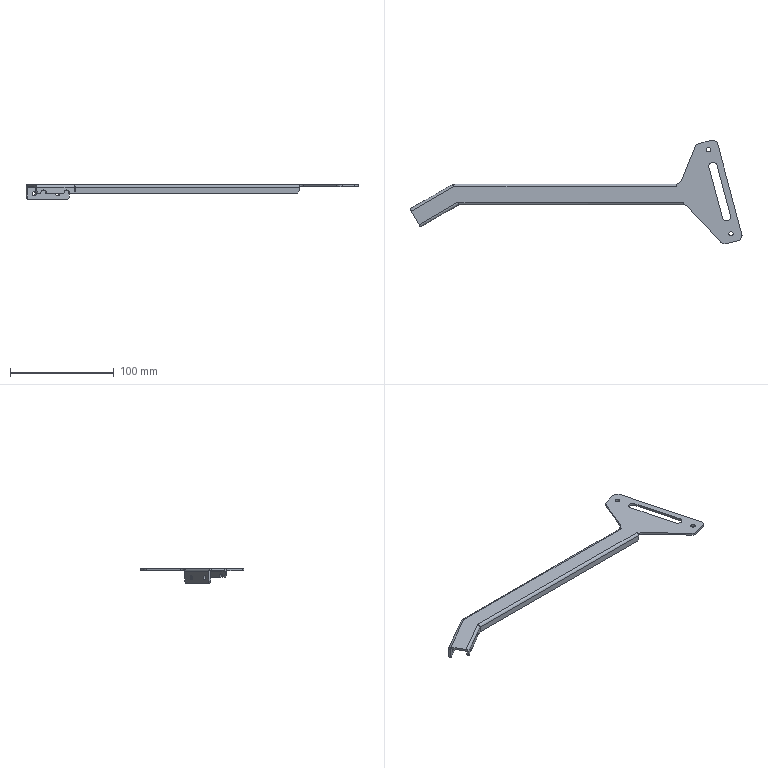Part | SolidWorks | features ICE 5, Chamfer 2, HoleWzd 2, 3DProfileFeature 1, EdgeFlange 1, Fillet 1, FlatPattern 1, SMBaseFlange 1, SheetMetal 1 | 1 solid | 75 faces | box 320.025 x 100.043 x 14 mm | volume 22575 mm3 | plane 43 | cylinder 28 | spline 4 | commonest cylinder face diameters 10 x7 1 x4 4.2 x4 4.5 x4 5 x4 8 x3